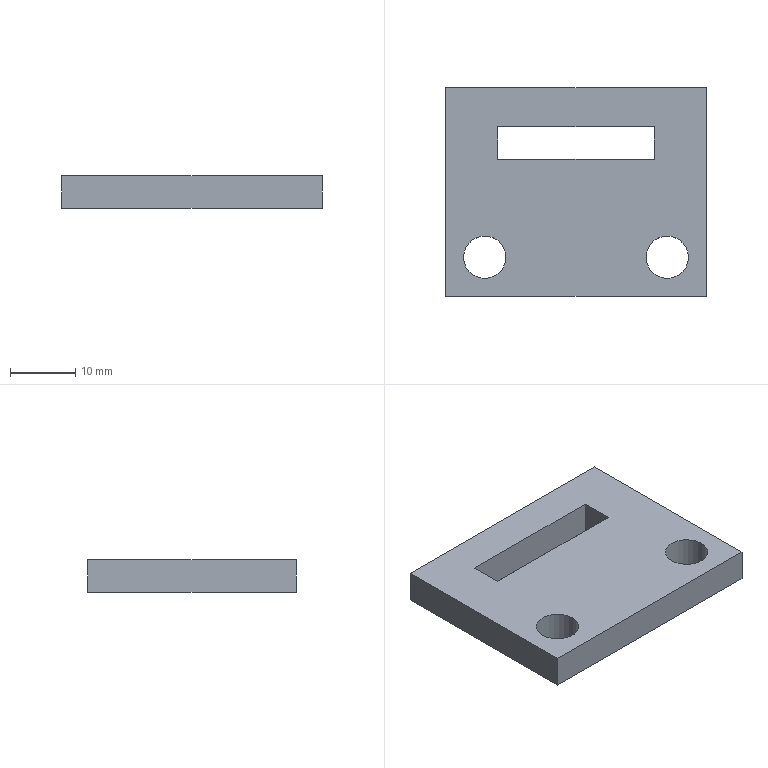Part | 1 solid | 14 faces | box 40 x 32 x 5 mm | volume 5295 mm3 | plane 10 | cylinder 4 | commonest cylinder face diameters 6.5 x4
STEP:
#1=CARTESIAN_POINT('',(10.75,0.,5.));
#2=VERTEX_POINT('',#1);
#3=CARTESIAN_POINT('',(17.25,0.,5.));
#4=VERTEX_POINT('',#3);
#5=CARTESIAN_POINT('',(14.,0.,5.));
#6=DIRECTION('',(0.,0.,1.));
#7=DIRECTION('',(1.,0.,0.));
#8=AXIS2_PLACEMENT_3D('',#5,#6,#7);
#9=CIRCLE('',#8,3.25);
#10=EDGE_CURVE('',#2,#4,#9,.T.);
#11=ORIENTED_EDGE('',*,*,#10,.T.);
#12=CARTESIAN_POINT('',(17.25,0.,0.));
#13=VERTEX_POINT('',#12);
#14=CARTESIAN_POINT('',(17.25,0.,5.));
#15=DIRECTION('',(0.,0.,-1.));
#16=VECTOR('',#15,1000.);
#17=LINE('',#14,#16);
#18=EDGE_CURVE('',#4,#13,#17,.T.);
#19=ORIENTED_EDGE('',*,*,#18,.T.);
#20=CARTESIAN_POINT('',(10.75,0.,0.));
#21=VERTEX_POINT('',#20);
#22=CARTESIAN_POINT('',(14.,0.,0.));
#23=DIRECTION('',(0.,0.,1.));
#24=DIRECTION('',(1.,0.,0.));
#25=AXIS2_PLACEMENT_3D('',#22,#23,#24);
#26=CIRCLE('',#25,3.25);
#27=EDGE_CURVE('',#21,#13,#26,.T.);
#28=ORIENTED_EDGE('',*,*,#27,.F.);
#29=CARTESIAN_POINT('',(10.75,0.,5.));
#30=DIRECTION('',(0.,0.,-1.));
#31=VECTOR('',#30,1000.);
#32=LINE('',#29,#31);
#33=EDGE_CURVE('',#2,#21,#32,.T.);
#34=ORIENTED_EDGE('',*,*,#33,.F.);
#35=EDGE_LOOP('',(#11,#19,#28,#34));
#36=FACE_OUTER_BOUND('',#35,.T.);
#37=CARTESIAN_POINT('',(14.,0.,5.));
#38=DIRECTION('',(0.,0.,-1.));
#39=DIRECTION('',(-1.,0.,0.));
#40=AXIS2_PLACEMENT_3D('',#37,#38,#39);
#41=CYLINDRICAL_SURFACE('',#40,3.25);
#42=ADVANCED_FACE('',(#36),#41,.F.);
#43=CARTESIAN_POINT('',(-17.25,0.,5.));
#44=VERTEX_POINT('',#43);
#45=CARTESIAN_POINT('',(-10.75,0.,5.));
#46=VERTEX_POINT('',#45);
#47=CARTESIAN_POINT('',(-14.,0.,5.));
#48=DIRECTION('',(0.,0.,1.));
#49=DIRECTION('',(1.,0.,0.));
#50=AXIS2_PLACEMENT_3D('',#47,#48,#49);
#51=CIRCLE('',#50,3.25);
#52=EDGE_CURVE('',#44,#46,#51,.T.);
#53=ORIENTED_EDGE('',*,*,#52,.T.);
#54=CARTESIAN_POINT('',(-10.75,0.,0.));
#55=VERTEX_POINT('',#54);
#56=CARTESIAN_POINT('',(-10.75,0.,5.));
#57=DIRECTION('',(0.,0.,-1.));
#58=VECTOR('',#57,1000.);
#59=LINE('',#56,#58);
#60=EDGE_CURVE('',#46,#55,#59,.T.);
#61=ORIENTED_EDGE('',*,*,#60,.T.);
#62=CARTESIAN_POINT('',(-17.25,0.,0.));
#63=VERTEX_POINT('',#62);
#64=CARTESIAN_POINT('',(-14.,0.,0.));
#65=DIRECTION('',(0.,0.,1.));
#66=DIRECTION('',(1.,0.,0.));
#67=AXIS2_PLACEMENT_3D('',#64,#65,#66);
#68=CIRCLE('',#67,3.25);
#69=EDGE_CURVE('',#63,#55,#68,.T.);
#70=ORIENTED_EDGE('',*,*,#69,.F.);
#71=CARTESIAN_POINT('',(-17.25,0.,5.));
#72=DIRECTION('',(0.,0.,-1.));
#73=VECTOR('',#72,1000.);
#74=LINE('',#71,#73);
#75=EDGE_CURVE('',#44,#63,#74,.T.);
#76=ORIENTED_EDGE('',*,*,#75,.F.);
#77=EDGE_LOOP('',(#53,#61,#70,#76));
#78=FACE_OUTER_BOUND('',#77,.T.);
#79=CARTESIAN_POINT('',(-14.,0.,5.));
#80=DIRECTION('',(0.,0.,-1.));
#81=DIRECTION('',(-1.,0.,0.));
#82=AXIS2_PLACEMENT_3D('',#79,#80,#81);
#83=CYLINDRICAL_SURFACE('',#82,3.25);
#84=ADVANCED_FACE('',(#78),#83,.F.);
#85=ORIENTED_EDGE('',*,*,#52,.F.);
#86=CARTESIAN_POINT('',(-14.,0.,5.));
#87=DIRECTION('',(0.,0.,1.));
#88=DIRECTION('',(1.,0.,0.));
#89=AXIS2_PLACEMENT_3D('',#86,#87,#88);
#90=CIRCLE('',#89,3.25);
#91=EDGE_CURVE('',#46,#44,#90,.T.);
#92=ORIENTED_EDGE('',*,*,#91,.F.);
#93=EDGE_LOOP('',(#85,#92));
#94=FACE_BOUND('',#93,.T.);
#95=CARTESIAN_POINT('',(20.,-6.,5.));
#96=VERTEX_POINT('',#95);
#97=CARTESIAN_POINT('',(20.,26.,5.));
#98=VERTEX_POINT('',#97);
#99=CARTESIAN_POINT('',(20.,-6.,5.));
#100=DIRECTION('',(0.,1.,0.));
#101=VECTOR('',#100,1000.);
#102=LINE('',#99,#101);
#103=EDGE_CURVE('',#96,#98,#102,.T.);
#104=ORIENTED_EDGE('',*,*,#103,.T.);
#105=CARTESIAN_POINT('',(-20.,26.,5.));
#106=VERTEX_POINT('',#105);
#107=CARTESIAN_POINT('',(-20.,26.,5.));
#108=DIRECTION('',(-1.,0.,0.));
#109=VECTOR('',#108,1000.);
#110=LINE('',#107,#109);
#111=EDGE_CURVE('',#98,#106,#110,.T.);
#112=ORIENTED_EDGE('',*,*,#111,.T.);
#113=CARTESIAN_POINT('',(-20.,-6.,5.));
#114=VERTEX_POINT('',#113);
#115=CARTESIAN_POINT('',(-20.,-6.,5.));
#116=DIRECTION('',(0.,-1.,0.));
#117=VECTOR('',#116,1000.);
#118=LINE('',#115,#117);
#119=EDGE_CURVE('',#106,#114,#118,.T.);
#120=ORIENTED_EDGE('',*,*,#119,.T.);
#121=CARTESIAN_POINT('',(-20.,-6.,5.));
#122=DIRECTION('',(1.,0.,0.));
#123=VECTOR('',#122,1000.);
#124=LINE('',#121,#123);
#125=EDGE_CURVE('',#114,#96,#124,.T.);
#126=ORIENTED_EDGE('',*,*,#125,.T.);
#127=EDGE_LOOP('',(#104,#112,#120,#126));
#128=FACE_OUTER_BOUND('',#127,.T.);
#129=ORIENTED_EDGE('',*,*,#10,.F.);
#130=CARTESIAN_POINT('',(14.,0.,5.));
#131=DIRECTION('',(0.,0.,1.));
#132=DIRECTION('',(1.,0.,0.));
#133=AXIS2_PLACEMENT_3D('',#130,#131,#132);
#134=CIRCLE('',#133,3.25);
#135=EDGE_CURVE('',#4,#2,#134,.T.);
#136=ORIENTED_EDGE('',*,*,#135,.F.);
#137=EDGE_LOOP('',(#129,#136));
#138=FACE_BOUND('',#137,.T.);
#139=CARTESIAN_POINT('',(-12.,15.,5.));
#140=VERTEX_POINT('',#139);
#141=CARTESIAN_POINT('',(12.,15.,5.));
#142=VERTEX_POINT('',#141);
#143=CARTESIAN_POINT('',(-12.,15.,5.));
#144=DIRECTION('',(1.,0.,0.));
#145=VECTOR('',#144,1000.);
#146=LINE('',#143,#145);
#147=EDGE_CURVE('',#140,#142,#146,.T.);
#148=ORIENTED_EDGE('',*,*,#147,.F.);
#149=CARTESIAN_POINT('',(-12.,20.,5.));
#150=VERTEX_POINT('',#149);
#151=CARTESIAN_POINT('',(-12.,20.,5.));
#152=DIRECTION('',(0.,-1.,0.));
#153=VECTOR('',#152,1000.);
#154=LINE('',#151,#153);
#155=EDGE_CURVE('',#150,#140,#154,.T.);
#156=ORIENTED_EDGE('',*,*,#155,.F.);
#157=CARTESIAN_POINT('',(12.,20.,5.));
#158=VERTEX_POINT('',#157);
#159=CARTESIAN_POINT('',(-12.,20.,5.));
#160=DIRECTION('',(-1.,0.,0.));
#161=VECTOR('',#160,1000.);
#162=LINE('',#159,#161);
#163=EDGE_CURVE('',#158,#150,#162,.T.);
#164=ORIENTED_EDGE('',*,*,#163,.F.);
#165=CARTESIAN_POINT('',(12.,20.,5.));
#166=DIRECTION('',(0.,1.,0.));
#167=VECTOR('',#166,1000.);
#168=LINE('',#165,#167);
#169=EDGE_CURVE('',#142,#158,#168,.T.);
#170=ORIENTED_EDGE('',*,*,#169,.F.);
#171=EDGE_LOOP('',(#148,#156,#164,#170));
#172=FACE_BOUND('',#171,.T.);
#173=CARTESIAN_POINT('',(0.,0.,5.));
#174=DIRECTION('',(0.,0.,-1.));
#175=DIRECTION('',(-1.,0.,0.));
#176=AXIS2_PLACEMENT_3D('',#173,#174,#175);
#177=PLANE('',#176);
#178=ADVANCED_FACE('',(#94,#128,#138,#172),#177,.F.);
#179=ORIENTED_EDGE('',*,*,#69,.T.);
#180=CARTESIAN_POINT('',(-14.,0.,0.));
#181=DIRECTION('',(0.,0.,1.));
#182=DIRECTION('',(1.,0.,0.));
#183=AXIS2_PLACEMENT_3D('',#180,#181,#182);
#184=CIRCLE('',#183,3.25);
#185=EDGE_CURVE('',#55,#63,#184,.T.);
#186=ORIENTED_EDGE('',*,*,#185,.T.);
#187=EDGE_LOOP('',(#179,#186));
#188=FACE_BOUND('',#187,.T.);
#189=CARTESIAN_POINT('',(20.,-6.,0.));
#190=VERTEX_POINT('',#189);
#191=CARTESIAN_POINT('',(20.,26.,0.));
#192=VERTEX_POINT('',#191);
#193=CARTESIAN_POINT('',(20.,-6.,0.));
#194=DIRECTION('',(0.,1.,0.));
#195=VECTOR('',#194,1000.);
#196=LINE('',#193,#195);
#197=EDGE_CURVE('',#190,#192,#196,.T.);
#198=ORIENTED_EDGE('',*,*,#197,.F.);
#199=CARTESIAN_POINT('',(-20.,-6.,0.));
#200=VERTEX_POINT('',#199);
#201=CARTESIAN_POINT('',(-20.,-6.,0.));
#202=DIRECTION('',(1.,0.,0.));
#203=VECTOR('',#202,1000.);
#204=LINE('',#201,#203);
#205=EDGE_CURVE('',#200,#190,#204,.T.);
#206=ORIENTED_EDGE('',*,*,#205,.F.);
#207=CARTESIAN_POINT('',(-20.,26.,0.));
#208=VERTEX_POINT('',#207);
#209=CARTESIAN_POINT('',(-20.,-6.,0.));
#210=DIRECTION('',(0.,-1.,0.));
#211=VECTOR('',#210,1000.);
#212=LINE('',#209,#211);
#213=EDGE_CURVE('',#208,#200,#212,.T.);
#214=ORIENTED_EDGE('',*,*,#213,.F.);
#215=CARTESIAN_POINT('',(-20.,26.,0.));
#216=DIRECTION('',(-1.,0.,0.));
#217=VECTOR('',#216,1000.);
#218=LINE('',#215,#217);
#219=EDGE_CURVE('',#192,#208,#218,.T.);
#220=ORIENTED_EDGE('',*,*,#219,.F.);
#221=EDGE_LOOP('',(#198,#206,#214,#220));
#222=FACE_OUTER_BOUND('',#221,.T.);
#223=ORIENTED_EDGE('',*,*,#27,.T.);
#224=CARTESIAN_POINT('',(14.,0.,0.));
#225=DIRECTION('',(0.,0.,1.));
#226=DIRECTION('',(1.,0.,0.));
#227=AXIS2_PLACEMENT_3D('',#224,#225,#226);
#228=CIRCLE('',#227,3.25);
#229=EDGE_CURVE('',#13,#21,#228,.T.);
#230=ORIENTED_EDGE('',*,*,#229,.T.);
#231=EDGE_LOOP('',(#223,#230));
#232=FACE_BOUND('',#231,.T.);
#233=CARTESIAN_POINT('',(-12.,12.113,0.));
#234=VERTEX_POINT('',#233);
#235=CARTESIAN_POINT('',(12.,12.113,0.));
#236=VERTEX_POINT('',#235);
#237=CARTESIAN_POINT('',(12.,12.113,0.));
#238=DIRECTION('',(1.,0.,0.));
#239=VECTOR('',#238,1000.);
#240=LINE('',#237,#239);
#241=EDGE_CURVE('',#234,#236,#240,.T.);
#242=ORIENTED_EDGE('',*,*,#241,.T.);
#243=CARTESIAN_POINT('',(12.,20.,0.));
#244=VERTEX_POINT('',#243);
#245=CARTESIAN_POINT('',(12.,20.,0.));
#246=DIRECTION('',(0.,1.,0.));
#247=VECTOR('',#246,1000.);
#248=LINE('',#245,#247);
#249=EDGE_CURVE('',#236,#244,#248,.T.);
#250=ORIENTED_EDGE('',*,*,#249,.T.);
#251=CARTESIAN_POINT('',(-12.,20.,0.));
#252=VERTEX_POINT('',#251);
#253=CARTESIAN_POINT('',(-12.,20.,0.));
#254=DIRECTION('',(-1.,0.,0.));
#255=VECTOR('',#254,1000.);
#256=LINE('',#253,#255);
#257=EDGE_CURVE('',#244,#252,#256,.T.);
#258=ORIENTED_EDGE('',*,*,#257,.T.);
#259=CARTESIAN_POINT('',(-12.,20.,0.));
#260=DIRECTION('',(0.,-1.,0.));
#261=VECTOR('',#260,1000.);
#262=LINE('',#259,#261);
#263=EDGE_CURVE('',#252,#234,#262,.T.);
#264=ORIENTED_EDGE('',*,*,#263,.T.);
#265=EDGE_LOOP('',(#242,#250,#258,#264));
#266=FACE_BOUND('',#265,.T.);
#267=CARTESIAN_POINT('',(0.,0.,0.));
#268=DIRECTION('',(0.,0.,-1.));
#269=DIRECTION('',(-1.,0.,0.));
#270=AXIS2_PLACEMENT_3D('',#267,#268,#269);
#271=PLANE('',#270);
#272=ADVANCED_FACE('',(#188,#222,#232,#266),#271,.T.);
#273=ORIENTED_EDGE('',*,*,#197,.T.);
#274=CARTESIAN_POINT('',(20.,26.,-44.721));
#275=DIRECTION('',(0.,0.,1.));
#276=VECTOR('',#275,1000.);
#277=LINE('',#274,#276);
#278=EDGE_CURVE('',#192,#98,#277,.T.);
#279=ORIENTED_EDGE('',*,*,#278,.T.);
#280=ORIENTED_EDGE('',*,*,#103,.F.);
#281=CARTESIAN_POINT('',(20.,-6.,5.));
#282=DIRECTION('',(0.,0.,-1.));
#283=VECTOR('',#282,1000.);
#284=LINE('',#281,#283);
#285=EDGE_CURVE('',#96,#190,#284,.T.);
#286=ORIENTED_EDGE('',*,*,#285,.T.);
#287=EDGE_LOOP('',(#273,#279,#280,#286));
#288=FACE_OUTER_BOUND('',#287,.T.);
#289=CARTESIAN_POINT('',(20.,-6.,5.));
#290=DIRECTION('',(-1.,0.,0.));
#291=DIRECTION('',(0.,0.,1.));
#292=AXIS2_PLACEMENT_3D('',#289,#290,#291);
#293=PLANE('',#292);
#294=ADVANCED_FACE('',(#288),#293,.F.);
#295=ORIENTED_EDGE('',*,*,#213,.T.);
#296=CARTESIAN_POINT('',(-20.,-6.,5.));
#297=DIRECTION('',(0.,0.,-1.));
#298=VECTOR('',#297,1000.);
#299=LINE('',#296,#298);
#300=EDGE_CURVE('',#114,#200,#299,.T.);
#301=ORIENTED_EDGE('',*,*,#300,.F.);
#302=ORIENTED_EDGE('',*,*,#119,.F.);
#303=CARTESIAN_POINT('',(-20.,26.,-44.721));
#304=DIRECTION('',(0.,0.,1.));
#305=VECTOR('',#304,1000.);
#306=LINE('',#303,#305);
#307=EDGE_CURVE('',#208,#106,#306,.T.);
#308=ORIENTED_EDGE('',*,*,#307,.F.);
#309=EDGE_LOOP('',(#295,#301,#302,#308));
#310=FACE_OUTER_BOUND('',#309,.T.);
#311=CARTESIAN_POINT('',(-20.,-6.,5.));
#312=DIRECTION('',(1.,0.,0.));
#313=DIRECTION('',(0.,0.,-1.));
#314=AXIS2_PLACEMENT_3D('',#311,#312,#313);
#315=PLANE('',#314);
#316=ADVANCED_FACE('',(#310),#315,.F.);
#317=ORIENTED_EDGE('',*,*,#205,.T.);
#318=ORIENTED_EDGE('',*,*,#285,.F.);
#319=ORIENTED_EDGE('',*,*,#125,.F.);
#320=ORIENTED_EDGE('',*,*,#300,.T.);
#321=EDGE_LOOP('',(#317,#318,#319,#320));
#322=FACE_OUTER_BOUND('',#321,.T.);
#323=CARTESIAN_POINT('',(-20.,-6.,5.));
#324=DIRECTION('',(0.,1.,0.));
#325=DIRECTION('',(0.,0.,1.));
#326=AXIS2_PLACEMENT_3D('',#323,#324,#325);
#327=PLANE('',#326);
#328=ADVANCED_FACE('',(#322),#327,.F.);
#329=ORIENTED_EDGE('',*,*,#60,.F.);
#330=ORIENTED_EDGE('',*,*,#91,.T.);
#331=ORIENTED_EDGE('',*,*,#75,.T.);
#332=ORIENTED_EDGE('',*,*,#185,.F.);
#333=EDGE_LOOP('',(#329,#330,#331,#332));
#334=FACE_OUTER_BOUND('',#333,.T.);
#335=CARTESIAN_POINT('',(-14.,0.,5.));
#336=DIRECTION('',(0.,0.,-1.));
#337=DIRECTION('',(-1.,0.,0.));
#338=AXIS2_PLACEMENT_3D('',#335,#336,#337);
#339=CYLINDRICAL_SURFACE('',#338,3.25);
#340=ADVANCED_FACE('',(#334),#339,.F.);
#341=ORIENTED_EDGE('',*,*,#18,.F.);
#342=ORIENTED_EDGE('',*,*,#135,.T.);
#343=ORIENTED_EDGE('',*,*,#33,.T.);
#344=ORIENTED_EDGE('',*,*,#229,.F.);
#345=EDGE_LOOP('',(#341,#342,#343,#344));
#346=FACE_OUTER_BOUND('',#345,.T.);
#347=CARTESIAN_POINT('',(14.,0.,5.));
#348=DIRECTION('',(0.,0.,-1.));
#349=DIRECTION('',(-1.,0.,0.));
#350=AXIS2_PLACEMENT_3D('',#347,#348,#349);
#351=CYLINDRICAL_SURFACE('',#350,3.25);
#352=ADVANCED_FACE('',(#346),#351,.F.);
#353=ORIENTED_EDGE('',*,*,#278,.F.);
#354=ORIENTED_EDGE('',*,*,#219,.T.);
#355=ORIENTED_EDGE('',*,*,#307,.T.);
#356=ORIENTED_EDGE('',*,*,#111,.F.);
#357=EDGE_LOOP('',(#353,#354,#355,#356));
#358=FACE_OUTER_BOUND('',#357,.T.);
#359=CARTESIAN_POINT('',(-20.,26.,-44.721));
#360=DIRECTION('',(0.,1.,0.));
#361=DIRECTION('',(0.,0.,1.));
#362=AXIS2_PLACEMENT_3D('',#359,#360,#361);
#363=PLANE('',#362);
#364=ADVANCED_FACE('',(#358),#363,.T.);
#365=ORIENTED_EDGE('',*,*,#263,.F.);
#366=CARTESIAN_POINT('',(-12.,20.,-44.721));
#367=DIRECTION('',(0.,0.,1.));
#368=VECTOR('',#367,1000.);
#369=LINE('',#366,#368);
#370=EDGE_CURVE('',#252,#150,#369,.T.);
#371=ORIENTED_EDGE('',*,*,#370,.T.);
#372=ORIENTED_EDGE('',*,*,#155,.T.);
#373=CARTESIAN_POINT('',(-12.,-5.28,-30.126));
#374=DIRECTION('',(0.,-0.5,-0.866));
#375=VECTOR('',#374,1000.);
#376=LINE('',#373,#375);
#377=EDGE_CURVE('',#140,#234,#376,.T.);
#378=ORIENTED_EDGE('',*,*,#377,.T.);
#379=EDGE_LOOP('',(#365,#371,#372,#378));
#380=FACE_OUTER_BOUND('',#379,.T.);
#381=CARTESIAN_POINT('',(-12.,20.,-44.721));
#382=DIRECTION('',(-1.,0.,0.));
#383=DIRECTION('',(0.,-1.,0.));
#384=AXIS2_PLACEMENT_3D('',#381,#382,#383);
#385=PLANE('',#384);
#386=ADVANCED_FACE('',(#380),#385,.F.);
#387=ORIENTED_EDGE('',*,*,#257,.F.);
#388=CARTESIAN_POINT('',(12.,20.,-44.721));
#389=DIRECTION('',(0.,0.,1.));
#390=VECTOR('',#389,1000.);
#391=LINE('',#388,#390);
#392=EDGE_CURVE('',#244,#158,#391,.T.);
#393=ORIENTED_EDGE('',*,*,#392,.T.);
#394=ORIENTED_EDGE('',*,*,#163,.T.);
#395=ORIENTED_EDGE('',*,*,#370,.F.);
#396=EDGE_LOOP('',(#387,#393,#394,#395));
#397=FACE_OUTER_BOUND('',#396,.T.);
#398=CARTESIAN_POINT('',(-12.,20.,-44.721));
#399=DIRECTION('',(0.,1.,0.));
#400=DIRECTION('',(0.,0.,1.));
#401=AXIS2_PLACEMENT_3D('',#398,#399,#400);
#402=PLANE('',#401);
#403=ADVANCED_FACE('',(#397),#402,.F.);
#404=ORIENTED_EDGE('',*,*,#249,.F.);
#405=CARTESIAN_POINT('',(12.,-5.28,-30.126));
#406=DIRECTION('',(0.,0.5,0.866));
#407=VECTOR('',#406,1000.);
#408=LINE('',#405,#407);
#409=EDGE_CURVE('',#236,#142,#408,.T.);
#410=ORIENTED_EDGE('',*,*,#409,.T.);
#411=ORIENTED_EDGE('',*,*,#169,.T.);
#412=ORIENTED_EDGE('',*,*,#392,.F.);
#413=EDGE_LOOP('',(#404,#410,#411,#412));
#414=FACE_OUTER_BOUND('',#413,.T.);
#415=CARTESIAN_POINT('',(12.,20.,-44.721));
#416=DIRECTION('',(1.,0.,0.));
#417=DIRECTION('',(0.,1.,0.));
#418=AXIS2_PLACEMENT_3D('',#415,#416,#417);
#419=PLANE('',#418);
#420=ADVANCED_FACE('',(#414),#419,.F.);
#421=ORIENTED_EDGE('',*,*,#377,.F.);
#422=ORIENTED_EDGE('',*,*,#147,.T.);
#423=ORIENTED_EDGE('',*,*,#409,.F.);
#424=ORIENTED_EDGE('',*,*,#241,.F.);
#425=EDGE_LOOP('',(#421,#422,#423,#424));
#426=FACE_OUTER_BOUND('',#425,.T.);
#427=CARTESIAN_POINT('',(0.,12.113,0.));
#428=DIRECTION('',(0.,0.866,-0.5));
#429=DIRECTION('',(-1.,0.,0.));
#430=AXIS2_PLACEMENT_3D('',#427,#428,#429);
#431=PLANE('',#430);
#432=ADVANCED_FACE('',(#426),#431,.T.);
#433=CLOSED_SHELL('',(#42,#84,#178,#272,#294,#316,#328,#340,#352,#364,#386,#403,#420,#432));
#434=MANIFOLD_SOLID_BREP('',#433);
#435=CARTESIAN_POINT('',(0.,0.,0.));
#436=DIRECTION('',(0.,0.,1.));
#437=DIRECTION('',(1.,0.,0.));
#438=AXIS2_PLACEMENT_3D('',#435,#436,#437);
#439=(LENGTH_UNIT()NAMED_UNIT(*)SI_UNIT(.MILLI.,.METRE.));
#440=UNCERTAINTY_MEASURE_WITH_UNIT(LENGTH_MEASURE(0.00001),#439,'','');
#441=(NAMED_UNIT(*)PLANE_ANGLE_UNIT()SI_UNIT($,.RADIAN.));
#442=(NAMED_UNIT(*)SI_UNIT($,.STERADIAN.)SOLID_ANGLE_UNIT());
#443=(GEOMETRIC_REPRESENTATION_CONTEXT(3)GLOBAL_UNCERTAINTY_ASSIGNED_CONTEXT((#440))GLOBAL_UNIT_ASSIGNED_CONTEXT((#439,#441,#442))REPRESENTATION_CONTEXT('',''));
#444=ADVANCED_BREP_SHAPE_REPRESENTATION('',(#434,#438),#443);